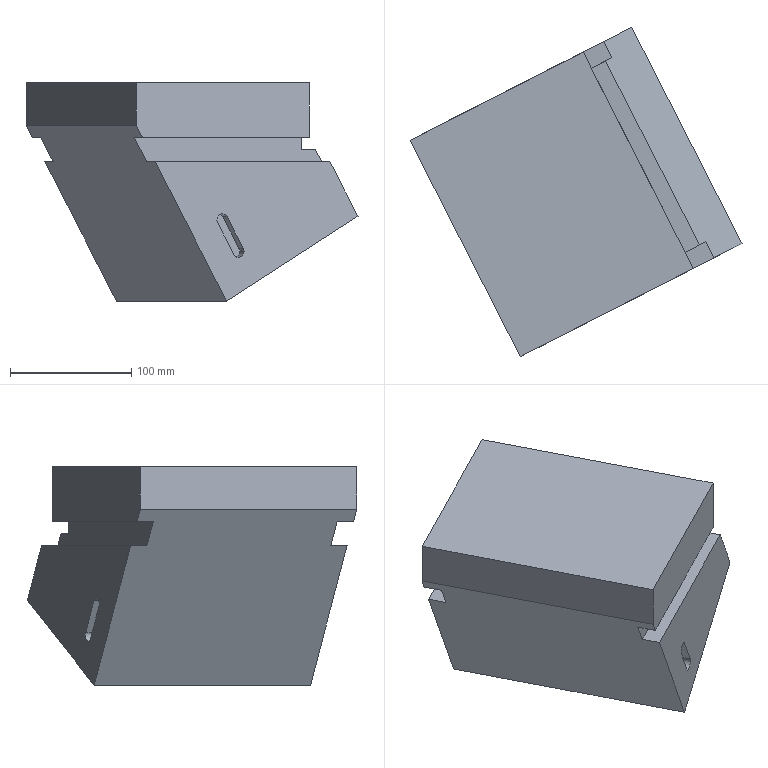Part | NX | features solid 2 | 1 solid | 27 faces | box 273.454 x 271.269 x 180 mm | volume 4546645 mm3 | plane 23 | cylinder 4 | commonest cylinder face diameters 10 x4
STEP:
#1=CARTESIAN_POINT('',(-1708.692,-455.362,180.));
#2=VERTEX_POINT('',#1);
#3=CARTESIAN_POINT('',(-1698.404,-450.119,160.));
#4=VERTEX_POINT('',#3);
#5=CARTESIAN_POINT('',(-1713.873,-458.001,190.07));
#6=DIRECTION('',(0.4455,0.227,-0.866));
#7=VECTOR('',#6,1000.);
#8=LINE('',#5,#7);
#9=EDGE_CURVE('',#2,#4,#8,.T.);
#10=ORIENTED_EDGE('',*,*,#9,.T.);
#11=CARTESIAN_POINT('',(-1705.214,-436.754,160.));
#12=VERTEX_POINT('',#11);
#13=CARTESIAN_POINT('',(-1614.416,-614.956,160.));
#14=DIRECTION('',(-0.454,0.891,0.));
#15=VECTOR('',#14,1000.);
#16=LINE('',#13,#15);
#17=EDGE_CURVE('',#4,#12,#16,.T.);
#18=ORIENTED_EDGE('',*,*,#17,.T.);
#19=CARTESIAN_POINT('',(-1646.055,-406.611,45.));
#20=VERTEX_POINT('',#19);
#21=CARTESIAN_POINT('',(-1720.683,-444.636,190.07));
#22=DIRECTION('',(0.4455,0.227,-0.866));
#23=VECTOR('',#22,1000.);
#24=LINE('',#21,#23);
#25=EDGE_CURVE('',#12,#20,#24,.T.);
#26=ORIENTED_EDGE('',*,*,#25,.T.);
#27=CARTESIAN_POINT('',(-1555.257,-584.813,45.));
#28=VERTEX_POINT('',#27);
#29=CARTESIAN_POINT('',(-1555.257,-584.813,45.));
#30=DIRECTION('',(-0.454,0.891,0.));
#31=VECTOR('',#30,1000.);
#32=LINE('',#29,#31);
#33=EDGE_CURVE('',#28,#20,#32,.T.);
#34=ORIENTED_EDGE('',*,*,#33,.F.);
#35=CARTESIAN_POINT('',(-1614.416,-614.956,160.));
#36=VERTEX_POINT('',#35);
#37=CARTESIAN_POINT('',(-1629.885,-622.837,190.07));
#38=DIRECTION('',(0.4455,0.227,-0.866));
#39=VECTOR('',#38,1000.);
#40=LINE('',#37,#39);
#41=EDGE_CURVE('',#36,#28,#40,.T.);
#42=ORIENTED_EDGE('',*,*,#41,.F.);
#43=CARTESIAN_POINT('',(-1621.226,-601.59,160.));
#44=VERTEX_POINT('',#43);
#45=CARTESIAN_POINT('',(-1614.416,-614.956,160.));
#46=DIRECTION('',(0.454,-0.891,0.));
#47=VECTOR('',#46,1000.);
#48=LINE('',#45,#47);
#49=EDGE_CURVE('',#44,#36,#48,.T.);
#50=ORIENTED_EDGE('',*,*,#49,.F.);
#51=CARTESIAN_POINT('',(-1631.514,-606.833,180.));
#52=VERTEX_POINT('',#51);
#53=CARTESIAN_POINT('',(-1636.694,-609.472,190.07));
#54=DIRECTION('',(0.4455,0.227,-0.866));
#55=VECTOR('',#54,1000.);
#56=LINE('',#53,#55);
#57=EDGE_CURVE('',#52,#44,#56,.T.);
#58=ORIENTED_EDGE('',*,*,#57,.F.);
#59=CARTESIAN_POINT('',(-1624.704,-620.198,180.));
#60=VERTEX_POINT('',#59);
#61=CARTESIAN_POINT('',(-1624.704,-620.198,180.));
#62=DIRECTION('',(0.454,-0.891,0.));
#63=VECTOR('',#62,1000.);
#64=LINE('',#61,#63);
#65=EDGE_CURVE('',#52,#60,#64,.T.);
#66=ORIENTED_EDGE('',*,*,#65,.T.);
#67=CARTESIAN_POINT('',(-1629.885,-622.837,190.07));
#68=VERTEX_POINT('',#67);
#69=CARTESIAN_POINT('',(-1629.885,-622.837,190.07));
#70=DIRECTION('',(0.4455,0.227,-0.866));
#71=VECTOR('',#70,1000.);
#72=LINE('',#69,#71);
#73=EDGE_CURVE('',#68,#60,#72,.T.);
#74=ORIENTED_EDGE('',*,*,#73,.F.);
#75=CARTESIAN_POINT('',(-1720.683,-444.636,190.07));
#76=VERTEX_POINT('',#75);
#77=CARTESIAN_POINT('',(-1629.885,-622.837,190.07));
#78=DIRECTION('',(-0.454,0.891,0.));
#79=VECTOR('',#78,1000.);
#80=LINE('',#77,#79);
#81=EDGE_CURVE('',#68,#76,#80,.T.);
#82=ORIENTED_EDGE('',*,*,#81,.T.);
#83=CARTESIAN_POINT('',(-1715.502,-441.996,180.));
#84=VERTEX_POINT('',#83);
#85=CARTESIAN_POINT('',(-1720.683,-444.636,190.07));
#86=DIRECTION('',(0.4455,0.227,-0.866));
#87=VECTOR('',#86,1000.);
#88=LINE('',#85,#87);
#89=EDGE_CURVE('',#76,#84,#88,.T.);
#90=ORIENTED_EDGE('',*,*,#89,.T.);
#91=CARTESIAN_POINT('',(-1624.704,-620.198,180.));
#92=DIRECTION('',(-0.454,0.891,0.));
#93=VECTOR('',#92,1000.);
#94=LINE('',#91,#93);
#95=EDGE_CURVE('',#2,#84,#94,.T.);
#96=ORIENTED_EDGE('',*,*,#95,.F.);
#97=EDGE_LOOP('',(#10,#18,#26,#34,#42,#50,#58,#66,#74,#82,#90,#96));
#98=FACE_BOUND('',#97,.T.);
#99=CARTESIAN_POINT('',(-1629.885,-622.837,190.07));
#100=DIRECTION('',(-0.7716,-0.3932,-0.5));
#101=DIRECTION('',(-0.4455,-0.227,0.866));
#102=AXIS2_PLACEMENT_3D('',#99,#100,#101);
#103=PLANE('',#102);
#104=ADVANCED_FACE('',(#98),#103,.T.);
#105=CARTESIAN_POINT('',(-1578.122,-371.998,180.));
#106=VERTEX_POINT('',#105);
#107=CARTESIAN_POINT('',(-1756.323,-462.796,180.));
#108=DIRECTION('',(0.891,0.454,0.));
#109=VECTOR('',#108,1000.);
#110=LINE('',#107,#109);
#111=EDGE_CURVE('',#84,#106,#110,.T.);
#112=ORIENTED_EDGE('',*,*,#111,.F.);
#113=ORIENTED_EDGE('',*,*,#89,.F.);
#114=CARTESIAN_POINT('',(-1720.683,-444.636,225.));
#115=VERTEX_POINT('',#114);
#116=CARTESIAN_POINT('',(-1720.683,-444.636,190.07));
#117=DIRECTION('',(0.,0.,1.));
#118=VECTOR('',#117,1000.);
#119=LINE('',#116,#118);
#120=EDGE_CURVE('',#76,#115,#119,.T.);
#121=ORIENTED_EDGE('',*,*,#120,.T.);
#122=CARTESIAN_POINT('',(-1578.122,-371.998,225.));
#123=VERTEX_POINT('',#122);
#124=CARTESIAN_POINT('',(-1720.683,-444.636,225.));
#125=DIRECTION('',(0.891,0.454,0.));
#126=VECTOR('',#125,1000.);
#127=LINE('',#124,#126);
#128=EDGE_CURVE('',#115,#123,#127,.T.);
#129=ORIENTED_EDGE('',*,*,#128,.T.);
#130=CARTESIAN_POINT('',(-1578.122,-371.998,170.));
#131=DIRECTION('',(0.,0.,1.));
#132=VECTOR('',#131,1000.);
#133=LINE('',#130,#132);
#134=EDGE_CURVE('',#106,#123,#133,.T.);
#135=ORIENTED_EDGE('',*,*,#134,.F.);
#136=EDGE_LOOP('',(#112,#113,#121,#129,#135));
#137=FACE_BOUND('',#136,.T.);
#138=CARTESIAN_POINT('',(-1720.683,-444.636,225.));
#139=DIRECTION('',(0.454,-0.891,0.));
#140=DIRECTION('',(0.,0.,1.));
#141=AXIS2_PLACEMENT_3D('',#138,#139,#140);
#142=PLANE('',#141);
#143=ADVANCED_FACE('',(#137),#142,.F.);
#144=CARTESIAN_POINT('',(-1571.312,-385.363,170.));
#145=VERTEX_POINT('',#144);
#146=CARTESIAN_POINT('',(-1571.312,-385.363,180.));
#147=VERTEX_POINT('',#146);
#148=CARTESIAN_POINT('',(-1571.312,-385.363,170.));
#149=DIRECTION('',(0.,0.,1.));
#150=VECTOR('',#149,1000.);
#151=LINE('',#148,#150);
#152=EDGE_CURVE('',#145,#147,#151,.T.);
#153=ORIENTED_EDGE('',*,*,#152,.T.);
#154=CARTESIAN_POINT('',(-1487.324,-550.199,180.));
#155=DIRECTION('',(0.454,-0.891,0.));
#156=VECTOR('',#155,1000.);
#157=LINE('',#154,#156);
#158=EDGE_CURVE('',#106,#147,#157,.T.);
#159=ORIENTED_EDGE('',*,*,#158,.F.);
#160=ORIENTED_EDGE('',*,*,#134,.T.);
#161=CARTESIAN_POINT('',(-1487.324,-550.199,225.));
#162=VERTEX_POINT('',#161);
#163=CARTESIAN_POINT('',(-1487.324,-550.199,225.));
#164=DIRECTION('',(-0.454,0.891,0.));
#165=VECTOR('',#164,1000.);
#166=LINE('',#163,#165);
#167=EDGE_CURVE('',#162,#123,#166,.T.);
#168=ORIENTED_EDGE('',*,*,#167,.F.);
#169=CARTESIAN_POINT('',(-1487.324,-550.199,180.));
#170=VERTEX_POINT('',#169);
#171=CARTESIAN_POINT('',(-1487.324,-550.199,170.));
#172=DIRECTION('',(0.,0.,1.));
#173=VECTOR('',#172,1000.);
#174=LINE('',#171,#173);
#175=EDGE_CURVE('',#170,#162,#174,.T.);
#176=ORIENTED_EDGE('',*,*,#175,.F.);
#177=CARTESIAN_POINT('',(-1494.133,-536.834,180.));
#178=VERTEX_POINT('',#177);
#179=CARTESIAN_POINT('',(-1487.324,-550.199,180.));
#180=DIRECTION('',(-0.454,0.891,0.));
#181=VECTOR('',#180,1000.);
#182=LINE('',#179,#181);
#183=EDGE_CURVE('',#170,#178,#182,.T.);
#184=ORIENTED_EDGE('',*,*,#183,.T.);
#185=CARTESIAN_POINT('',(-1494.133,-536.834,170.));
#186=VERTEX_POINT('',#185);
#187=CARTESIAN_POINT('',(-1494.133,-536.834,170.));
#188=DIRECTION('',(0.,0.,1.));
#189=VECTOR('',#188,1000.);
#190=LINE('',#187,#189);
#191=EDGE_CURVE('',#186,#178,#190,.T.);
#192=ORIENTED_EDGE('',*,*,#191,.F.);
#193=CARTESIAN_POINT('',(-1487.324,-550.199,170.));
#194=DIRECTION('',(-0.454,0.891,0.));
#195=VECTOR('',#194,1000.);
#196=LINE('',#193,#195);
#197=EDGE_CURVE('',#186,#145,#196,.T.);
#198=ORIENTED_EDGE('',*,*,#197,.T.);
#199=EDGE_LOOP('',(#153,#159,#160,#168,#176,#184,#192,#198));
#200=FACE_BOUND('',#199,.T.);
#201=CARTESIAN_POINT('',(-1487.324,-550.199,170.));
#202=DIRECTION('',(0.891,0.454,0.));
#203=DIRECTION('',(0.,0.,-1.));
#204=AXIS2_PLACEMENT_3D('',#201,#202,#203);
#205=PLANE('',#204);
#206=ADVANCED_FACE('',(#200),#205,.T.);
#207=CARTESIAN_POINT('',(-1559.51,-379.349,170.));
#208=VERTEX_POINT('',#207);
#209=CARTESIAN_POINT('',(-1559.51,-379.349,170.));
#210=DIRECTION('',(-0.891,-0.454,0.));
#211=VECTOR('',#210,1000.);
#212=LINE('',#209,#211);
#213=EDGE_CURVE('',#208,#145,#212,.T.);
#214=ORIENTED_EDGE('',*,*,#213,.T.);
#215=ORIENTED_EDGE('',*,*,#197,.F.);
#216=CARTESIAN_POINT('',(-1482.331,-530.82,170.));
#217=VERTEX_POINT('',#216);
#218=CARTESIAN_POINT('',(-1482.331,-530.82,170.));
#219=DIRECTION('',(-0.891,-0.454,0.));
#220=VECTOR('',#219,1000.);
#221=LINE('',#218,#220);
#222=EDGE_CURVE('',#217,#186,#221,.T.);
#223=ORIENTED_EDGE('',*,*,#222,.F.);
#224=CARTESIAN_POINT('',(-1475.521,-544.185,170.));
#225=DIRECTION('',(-0.454,0.891,0.));
#226=VECTOR('',#225,1000.);
#227=LINE('',#224,#226);
#228=EDGE_CURVE('',#217,#208,#227,.T.);
#229=ORIENTED_EDGE('',*,*,#228,.T.);
#230=EDGE_LOOP('',(#214,#215,#223,#229));
#231=FACE_BOUND('',#230,.T.);
#232=CARTESIAN_POINT('',(-1475.521,-544.185,170.));
#233=DIRECTION('',(0.,0.,1.));
#234=DIRECTION('',(0.891,0.454,0.));
#235=AXIS2_PLACEMENT_3D('',#232,#233,#234);
#236=PLANE('',#235);
#237=ADVANCED_FACE('',(#231),#236,.T.);
#238=CARTESIAN_POINT('',(-1554.365,-376.728,160.));
#239=VERTEX_POINT('',#238);
#240=CARTESIAN_POINT('',(-1531.216,-364.933,115.));
#241=DIRECTION('',(-0.4455,-0.227,0.866));
#242=VECTOR('',#241,1000.);
#243=LINE('',#240,#242);
#244=EDGE_CURVE('',#239,#208,#243,.T.);
#245=ORIENTED_EDGE('',*,*,#244,.T.);
#246=ORIENTED_EDGE('',*,*,#228,.F.);
#247=CARTESIAN_POINT('',(-1477.187,-528.199,160.));
#248=VERTEX_POINT('',#247);
#249=CARTESIAN_POINT('',(-1454.038,-516.404,115.));
#250=DIRECTION('',(-0.4455,-0.227,0.866));
#251=VECTOR('',#250,1000.);
#252=LINE('',#249,#251);
#253=EDGE_CURVE('',#248,#217,#252,.T.);
#254=ORIENTED_EDGE('',*,*,#253,.F.);
#255=CARTESIAN_POINT('',(-1470.377,-541.564,160.));
#256=VERTEX_POINT('',#255);
#257=CARTESIAN_POINT('',(-1470.377,-541.564,160.));
#258=DIRECTION('',(-0.454,0.891,0.));
#259=VECTOR('',#258,1000.);
#260=LINE('',#257,#259);
#261=EDGE_CURVE('',#256,#248,#260,.T.);
#262=ORIENTED_EDGE('',*,*,#261,.F.);
#263=CARTESIAN_POINT('',(-1447.228,-529.769,115.));
#264=VERTEX_POINT('',#263);
#265=CARTESIAN_POINT('',(-1447.228,-529.769,115.));
#266=DIRECTION('',(-0.4455,-0.227,0.866));
#267=VECTOR('',#266,1000.);
#268=LINE('',#265,#267);
#269=EDGE_CURVE('',#264,#256,#268,.T.);
#270=ORIENTED_EDGE('',*,*,#269,.F.);
#271=CARTESIAN_POINT('',(-1538.026,-351.568,115.));
#272=VERTEX_POINT('',#271);
#273=CARTESIAN_POINT('',(-1447.228,-529.769,115.));
#274=DIRECTION('',(-0.454,0.891,0.));
#275=VECTOR('',#274,1000.);
#276=LINE('',#273,#275);
#277=EDGE_CURVE('',#264,#272,#276,.T.);
#278=ORIENTED_EDGE('',*,*,#277,.T.);
#279=CARTESIAN_POINT('',(-1561.175,-363.363,160.));
#280=VERTEX_POINT('',#279);
#281=CARTESIAN_POINT('',(-1538.026,-351.568,115.));
#282=DIRECTION('',(-0.4455,-0.227,0.866));
#283=VECTOR('',#282,1000.);
#284=LINE('',#281,#283);
#285=EDGE_CURVE('',#272,#280,#284,.T.);
#286=ORIENTED_EDGE('',*,*,#285,.T.);
#287=CARTESIAN_POINT('',(-1470.377,-541.564,160.));
#288=DIRECTION('',(0.454,-0.891,0.));
#289=VECTOR('',#288,1000.);
#290=LINE('',#287,#289);
#291=EDGE_CURVE('',#280,#239,#290,.T.);
#292=ORIENTED_EDGE('',*,*,#291,.T.);
#293=EDGE_LOOP('',(#245,#246,#254,#262,#270,#278,#286,#292));
#294=FACE_BOUND('',#293,.T.);
#295=CARTESIAN_POINT('',(-1447.228,-529.769,115.));
#296=DIRECTION('',(0.7716,0.3932,0.5));
#297=DIRECTION('',(0.4455,0.227,-0.866));
#298=AXIS2_PLACEMENT_3D('',#295,#296,#297);
#299=PLANE('',#298);
#300=ADVANCED_FACE('',(#294),#299,.T.);
#301=CARTESIAN_POINT('',(-1541.701,-577.905,88.647));
#302=VERTEX_POINT('',#301);
#303=CARTESIAN_POINT('',(-1555.066,-584.715,114.628));
#304=VERTEX_POINT('',#303);
#305=CARTESIAN_POINT('',(-1548.383,-581.31,101.638));
#306=DIRECTION('',(-0.4455,-0.227,0.866));
#307=VECTOR('',#306,1000.);
#308=LINE('',#305,#307);
#309=EDGE_CURVE('',#302,#304,#308,.T.);
#310=ORIENTED_EDGE('',*,*,#309,.F.);
#311=CARTESIAN_POINT('',(-1549.417,-581.837,83.647));
#312=VERTEX_POINT('',#311);
#313=CARTESIAN_POINT('',(-1545.559,-579.871,86.147));
#314=DIRECTION('',(-0.454,0.891,0.));
#315=DIRECTION('',(0.,0.,1.));
#316=AXIS2_PLACEMENT_3D('',#313,#314,#315);
#317=CIRCLE('',#316,5.);
#318=EDGE_CURVE('',#302,#312,#317,.T.);
#319=ORIENTED_EDGE('',*,*,#318,.T.);
#320=CARTESIAN_POINT('',(-1562.782,-588.647,109.628));
#321=VERTEX_POINT('',#320);
#322=CARTESIAN_POINT('',(-1556.1,-585.242,96.638));
#323=DIRECTION('',(-0.4455,-0.227,0.866));
#324=VECTOR('',#323,1000.);
#325=LINE('',#322,#324);
#326=EDGE_CURVE('',#312,#321,#325,.T.);
#327=ORIENTED_EDGE('',*,*,#326,.T.);
#328=CARTESIAN_POINT('',(-1558.924,-586.681,112.128));
#329=DIRECTION('',(-0.454,0.891,0.));
#330=DIRECTION('',(0.,0.,1.));
#331=AXIS2_PLACEMENT_3D('',#328,#329,#330);
#332=CIRCLE('',#331,5.);
#333=EDGE_CURVE('',#321,#304,#332,.T.);
#334=ORIENTED_EDGE('',*,*,#333,.T.);
#335=EDGE_LOOP('',(#310,#319,#327,#334));
#336=FACE_BOUND('',#335,.T.);
#337=ORIENTED_EDGE('',*,*,#41,.T.);
#338=CARTESIAN_POINT('',(-1447.228,-529.769,115.));
#339=DIRECTION('',(-0.7716,-0.3932,-0.5));
#340=VECTOR('',#339,1000.);
#341=LINE('',#338,#340);
#342=EDGE_CURVE('',#264,#28,#341,.T.);
#343=ORIENTED_EDGE('',*,*,#342,.F.);
#344=ORIENTED_EDGE('',*,*,#269,.T.);
#345=CARTESIAN_POINT('',(-1665.525,-640.997,160.));
#346=DIRECTION('',(0.891,0.454,0.));
#347=VECTOR('',#346,1000.);
#348=LINE('',#345,#347);
#349=EDGE_CURVE('',#36,#256,#348,.T.);
#350=ORIENTED_EDGE('',*,*,#349,.F.);
#351=EDGE_LOOP('',(#337,#343,#344,#350));
#352=FACE_BOUND('',#351,.T.);
#353=CARTESIAN_POINT('',(-1629.885,-622.837,225.));
#354=DIRECTION('',(0.454,-0.891,0.));
#355=DIRECTION('',(0.,0.,1.));
#356=AXIS2_PLACEMENT_3D('',#353,#354,#355);
#357=PLANE('',#356);
#358=ADVANCED_FACE('',(#336,#352),#357,.T.);
#359=ORIENTED_EDGE('',*,*,#120,.F.);
#360=ORIENTED_EDGE('',*,*,#81,.F.);
#361=CARTESIAN_POINT('',(-1629.885,-622.837,225.));
#362=VERTEX_POINT('',#361);
#363=CARTESIAN_POINT('',(-1629.885,-622.837,190.07));
#364=DIRECTION('',(0.,0.,1.));
#365=VECTOR('',#364,1000.);
#366=LINE('',#363,#365);
#367=EDGE_CURVE('',#68,#362,#366,.T.);
#368=ORIENTED_EDGE('',*,*,#367,.T.);
#369=CARTESIAN_POINT('',(-1629.885,-622.837,225.));
#370=DIRECTION('',(-0.454,0.891,0.));
#371=VECTOR('',#370,1000.);
#372=LINE('',#369,#371);
#373=EDGE_CURVE('',#362,#115,#372,.T.);
#374=ORIENTED_EDGE('',*,*,#373,.T.);
#375=EDGE_LOOP('',(#359,#360,#368,#374));
#376=FACE_BOUND('',#375,.T.);
#377=CARTESIAN_POINT('',(-1629.885,-622.837,190.07));
#378=DIRECTION('',(0.891,0.454,0.));
#379=DIRECTION('',(0.,0.,-1.));
#380=AXIS2_PLACEMENT_3D('',#377,#378,#379);
#381=PLANE('',#380);
#382=ADVANCED_FACE('',(#376),#381,.F.);
#383=ORIENTED_EDGE('',*,*,#128,.F.);
#384=ORIENTED_EDGE('',*,*,#373,.F.);
#385=CARTESIAN_POINT('',(-1629.885,-622.837,225.));
#386=DIRECTION('',(0.891,0.454,0.));
#387=VECTOR('',#386,1000.);
#388=LINE('',#385,#387);
#389=EDGE_CURVE('',#362,#162,#388,.T.);
#390=ORIENTED_EDGE('',*,*,#389,.T.);
#391=ORIENTED_EDGE('',*,*,#167,.T.);
#392=EDGE_LOOP('',(#383,#384,#390,#391));
#393=FACE_BOUND('',#392,.T.);
#394=CARTESIAN_POINT('',(-1629.885,-622.837,225.));
#395=DIRECTION('',(0.,0.,-1.));
#396=DIRECTION('',(-0.891,-0.454,0.));
#397=AXIS2_PLACEMENT_3D('',#394,#395,#396);
#398=PLANE('',#397);
#399=ADVANCED_FACE('',(#393),#398,.F.);
#400=CARTESIAN_POINT('',(-1538.026,-351.568,115.));
#401=DIRECTION('',(-0.7716,-0.3932,-0.5));
#402=VECTOR('',#401,1000.);
#403=LINE('',#400,#402);
#404=EDGE_CURVE('',#272,#20,#403,.T.);
#405=ORIENTED_EDGE('',*,*,#404,.F.);
#406=ORIENTED_EDGE('',*,*,#277,.F.);
#407=ORIENTED_EDGE('',*,*,#342,.T.);
#408=ORIENTED_EDGE('',*,*,#33,.T.);
#409=EDGE_LOOP('',(#405,#406,#407,#408));
#410=FACE_BOUND('',#409,.T.);
#411=CARTESIAN_POINT('',(-1447.228,-529.769,115.));
#412=DIRECTION('',(-0.4455,-0.227,0.866));
#413=DIRECTION('',(0.7716,0.3932,0.5));
#414=AXIS2_PLACEMENT_3D('',#411,#412,#413);
#415=PLANE('',#414);
#416=ADVANCED_FACE('',(#410),#415,.F.);
#417=CARTESIAN_POINT('',(-1665.525,-640.997,180.));
#418=DIRECTION('',(0.891,0.454,0.));
#419=VECTOR('',#418,1000.);
#420=LINE('',#417,#419);
#421=EDGE_CURVE('',#60,#170,#420,.T.);
#422=ORIENTED_EDGE('',*,*,#421,.T.);
#423=ORIENTED_EDGE('',*,*,#175,.T.);
#424=ORIENTED_EDGE('',*,*,#389,.F.);
#425=ORIENTED_EDGE('',*,*,#367,.F.);
#426=ORIENTED_EDGE('',*,*,#73,.T.);
#427=EDGE_LOOP('',(#422,#423,#424,#425,#426));
#428=FACE_BOUND('',#427,.T.);
#429=CARTESIAN_POINT('',(-1629.885,-622.837,225.));
#430=DIRECTION('',(0.454,-0.891,0.));
#431=DIRECTION('',(0.,0.,1.));
#432=AXIS2_PLACEMENT_3D('',#429,#430,#431);
#433=PLANE('',#432);
#434=ADVANCED_FACE('',(#428),#433,.T.);
#435=CARTESIAN_POINT('',(-1645.864,-406.514,114.628));
#436=VERTEX_POINT('',#435);
#437=CARTESIAN_POINT('',(-1653.58,-410.446,109.628));
#438=VERTEX_POINT('',#437);
#439=CARTESIAN_POINT('',(-1649.722,-408.48,112.128));
#440=DIRECTION('',(0.454,-0.891,0.));
#441=DIRECTION('',(0.,0.,-1.));
#442=AXIS2_PLACEMENT_3D('',#439,#440,#441);
#443=CIRCLE('',#442,5.);
#444=EDGE_CURVE('',#436,#438,#443,.T.);
#445=ORIENTED_EDGE('',*,*,#444,.T.);
#446=CARTESIAN_POINT('',(-1640.215,-403.636,83.647));
#447=VERTEX_POINT('',#446);
#448=CARTESIAN_POINT('',(-1646.898,-407.041,96.638));
#449=DIRECTION('',(0.4455,0.227,-0.866));
#450=VECTOR('',#449,1000.);
#451=LINE('',#448,#450);
#452=EDGE_CURVE('',#438,#447,#451,.T.);
#453=ORIENTED_EDGE('',*,*,#452,.T.);
#454=CARTESIAN_POINT('',(-1632.499,-399.704,88.647));
#455=VERTEX_POINT('',#454);
#456=CARTESIAN_POINT('',(-1636.357,-401.67,86.147));
#457=DIRECTION('',(0.454,-0.891,0.));
#458=DIRECTION('',(0.,0.,-1.));
#459=AXIS2_PLACEMENT_3D('',#456,#457,#458);
#460=CIRCLE('',#459,5.);
#461=EDGE_CURVE('',#447,#455,#460,.T.);
#462=ORIENTED_EDGE('',*,*,#461,.T.);
#463=CARTESIAN_POINT('',(-1639.181,-403.109,101.638));
#464=DIRECTION('',(0.4455,0.227,-0.866));
#465=VECTOR('',#464,1000.);
#466=LINE('',#463,#465);
#467=EDGE_CURVE('',#436,#455,#466,.T.);
#468=ORIENTED_EDGE('',*,*,#467,.F.);
#469=EDGE_LOOP('',(#445,#453,#462,#468));
#470=FACE_BOUND('',#469,.T.);
#471=ORIENTED_EDGE('',*,*,#285,.F.);
#472=ORIENTED_EDGE('',*,*,#404,.T.);
#473=ORIENTED_EDGE('',*,*,#25,.F.);
#474=CARTESIAN_POINT('',(-1756.323,-462.796,160.));
#475=DIRECTION('',(0.891,0.454,0.));
#476=VECTOR('',#475,1000.);
#477=LINE('',#474,#476);
#478=EDGE_CURVE('',#12,#280,#477,.T.);
#479=ORIENTED_EDGE('',*,*,#478,.T.);
#480=EDGE_LOOP('',(#471,#472,#473,#479));
#481=FACE_BOUND('',#480,.T.);
#482=CARTESIAN_POINT('',(-1720.683,-444.636,225.));
#483=DIRECTION('',(0.454,-0.891,0.));
#484=DIRECTION('',(0.,0.,1.));
#485=AXIS2_PLACEMENT_3D('',#482,#483,#484);
#486=PLANE('',#485);
#487=ADVANCED_FACE('',(#470,#481),#486,.F.);
#488=ORIENTED_EDGE('',*,*,#467,.T.);
#489=CARTESIAN_POINT('',(-1628.867,-406.832,88.647));
#490=VERTEX_POINT('',#489);
#491=CARTESIAN_POINT('',(-1632.499,-399.704,88.647));
#492=DIRECTION('',(-0.454,0.891,0.));
#493=VECTOR('',#492,1000.);
#494=LINE('',#491,#493);
#495=EDGE_CURVE('',#490,#455,#494,.T.);
#496=ORIENTED_EDGE('',*,*,#495,.F.);
#497=CARTESIAN_POINT('',(-1642.232,-413.642,114.628));
#498=VERTEX_POINT('',#497);
#499=CARTESIAN_POINT('',(-1642.232,-413.642,114.628));
#500=DIRECTION('',(0.4455,0.227,-0.866));
#501=VECTOR('',#500,1000.);
#502=LINE('',#499,#501);
#503=EDGE_CURVE('',#498,#490,#502,.T.);
#504=ORIENTED_EDGE('',*,*,#503,.F.);
#505=CARTESIAN_POINT('',(-1645.864,-406.514,114.628));
#506=DIRECTION('',(-0.454,0.891,0.));
#507=VECTOR('',#506,1000.);
#508=LINE('',#505,#507);
#509=EDGE_CURVE('',#498,#436,#508,.T.);
#510=ORIENTED_EDGE('',*,*,#509,.T.);
#511=EDGE_LOOP('',(#488,#496,#504,#510));
#512=FACE_BOUND('',#511,.T.);
#513=CARTESIAN_POINT('',(-1639.181,-403.109,101.638));
#514=DIRECTION('',(0.7716,0.3932,0.5));
#515=DIRECTION('',(0.4455,0.227,-0.866));
#516=AXIS2_PLACEMENT_3D('',#513,#514,#515);
#517=PLANE('',#516);
#518=ADVANCED_FACE('',(#512),#517,.F.);
#519=ORIENTED_EDGE('',*,*,#503,.T.);
#520=CARTESIAN_POINT('',(-1636.583,-410.764,83.647));
#521=VERTEX_POINT('',#520);
#522=CARTESIAN_POINT('',(-1632.725,-408.798,86.147));
#523=DIRECTION('',(0.454,-0.891,0.));
#524=DIRECTION('',(0.,0.,-1.));
#525=AXIS2_PLACEMENT_3D('',#522,#523,#524);
#526=CIRCLE('',#525,5.);
#527=EDGE_CURVE('',#521,#490,#526,.T.);
#528=ORIENTED_EDGE('',*,*,#527,.F.);
#529=CARTESIAN_POINT('',(-1649.948,-417.574,109.628));
#530=VERTEX_POINT('',#529);
#531=CARTESIAN_POINT('',(-1649.948,-417.574,109.628));
#532=DIRECTION('',(0.4455,0.227,-0.866));
#533=VECTOR('',#532,1000.);
#534=LINE('',#531,#533);
#535=EDGE_CURVE('',#530,#521,#534,.T.);
#536=ORIENTED_EDGE('',*,*,#535,.F.);
#537=CARTESIAN_POINT('',(-1646.09,-415.608,112.128));
#538=DIRECTION('',(0.454,-0.891,0.));
#539=DIRECTION('',(0.,0.,-1.));
#540=AXIS2_PLACEMENT_3D('',#537,#538,#539);
#541=CIRCLE('',#540,5.);
#542=EDGE_CURVE('',#498,#530,#541,.T.);
#543=ORIENTED_EDGE('',*,*,#542,.F.);
#544=EDGE_LOOP('',(#519,#528,#536,#543));
#545=FACE_BOUND('',#544,.T.);
#546=CARTESIAN_POINT('',(-1639.408,-412.203,99.138));
#547=DIRECTION('',(0.454,-0.891,0.));
#548=DIRECTION('',(0.,0.,1.));
#549=AXIS2_PLACEMENT_3D('',#546,#547,#548);
#550=PLANE('',#549);
#551=ADVANCED_FACE('',(#545),#550,.F.);
#552=ORIENTED_EDGE('',*,*,#444,.F.);
#553=ORIENTED_EDGE('',*,*,#509,.F.);
#554=ORIENTED_EDGE('',*,*,#542,.T.);
#555=CARTESIAN_POINT('',(-1653.58,-410.446,109.628));
#556=DIRECTION('',(-0.454,0.891,0.));
#557=VECTOR('',#556,1000.);
#558=LINE('',#555,#557);
#559=EDGE_CURVE('',#530,#438,#558,.T.);
#560=ORIENTED_EDGE('',*,*,#559,.T.);
#561=EDGE_LOOP('',(#552,#553,#554,#560));
#562=FACE_BOUND('',#561,.T.);
#563=CARTESIAN_POINT('',(-1649.722,-408.48,112.128));
#564=DIRECTION('',(-0.454,0.891,0.));
#565=DIRECTION('',(0.,0.,-1.));
#566=AXIS2_PLACEMENT_3D('',#563,#564,#565);
#567=CYLINDRICAL_SURFACE('',#566,5.);
#568=ADVANCED_FACE('',(#562),#567,.F.);
#569=ORIENTED_EDGE('',*,*,#452,.F.);
#570=ORIENTED_EDGE('',*,*,#559,.F.);
#571=ORIENTED_EDGE('',*,*,#535,.T.);
#572=CARTESIAN_POINT('',(-1640.215,-403.636,83.647));
#573=DIRECTION('',(-0.454,0.891,0.));
#574=VECTOR('',#573,1000.);
#575=LINE('',#572,#574);
#576=EDGE_CURVE('',#521,#447,#575,.T.);
#577=ORIENTED_EDGE('',*,*,#576,.T.);
#578=EDGE_LOOP('',(#569,#570,#571,#577));
#579=FACE_BOUND('',#578,.T.);
#580=CARTESIAN_POINT('',(-1646.898,-407.041,96.638));
#581=DIRECTION('',(-0.7716,-0.3932,-0.5));
#582=DIRECTION('',(-0.4455,-0.227,0.866));
#583=AXIS2_PLACEMENT_3D('',#580,#581,#582);
#584=PLANE('',#583);
#585=ADVANCED_FACE('',(#579),#584,.F.);
#586=ORIENTED_EDGE('',*,*,#461,.F.);
#587=ORIENTED_EDGE('',*,*,#576,.F.);
#588=ORIENTED_EDGE('',*,*,#527,.T.);
#589=ORIENTED_EDGE('',*,*,#495,.T.);
#590=EDGE_LOOP('',(#586,#587,#588,#589));
#591=FACE_BOUND('',#590,.T.);
#592=CARTESIAN_POINT('',(-1636.357,-401.67,86.147));
#593=DIRECTION('',(-0.454,0.891,0.));
#594=DIRECTION('',(0.,0.,-1.));
#595=AXIS2_PLACEMENT_3D('',#592,#593,#594);
#596=CYLINDRICAL_SURFACE('',#595,5.);
#597=ADVANCED_FACE('',(#591),#596,.F.);
#598=ORIENTED_EDGE('',*,*,#309,.T.);
#599=CARTESIAN_POINT('',(-1558.698,-577.587,114.628));
#600=VERTEX_POINT('',#599);
#601=CARTESIAN_POINT('',(-1555.066,-584.715,114.628));
#602=DIRECTION('',(0.454,-0.891,0.));
#603=VECTOR('',#602,1000.);
#604=LINE('',#601,#603);
#605=EDGE_CURVE('',#600,#304,#604,.T.);
#606=ORIENTED_EDGE('',*,*,#605,.F.);
#607=CARTESIAN_POINT('',(-1545.333,-570.777,88.647));
#608=VERTEX_POINT('',#607);
#609=CARTESIAN_POINT('',(-1545.333,-570.777,88.647));
#610=DIRECTION('',(-0.4455,-0.227,0.866));
#611=VECTOR('',#610,1000.);
#612=LINE('',#609,#611);
#613=EDGE_CURVE('',#608,#600,#612,.T.);
#614=ORIENTED_EDGE('',*,*,#613,.F.);
#615=CARTESIAN_POINT('',(-1541.701,-577.905,88.647));
#616=DIRECTION('',(0.454,-0.891,0.));
#617=VECTOR('',#616,1000.);
#618=LINE('',#615,#617);
#619=EDGE_CURVE('',#608,#302,#618,.T.);
#620=ORIENTED_EDGE('',*,*,#619,.T.);
#621=EDGE_LOOP('',(#598,#606,#614,#620));
#622=FACE_BOUND('',#621,.T.);
#623=CARTESIAN_POINT('',(-1548.383,-581.31,101.638));
#624=DIRECTION('',(0.7716,0.3932,0.5));
#625=DIRECTION('',(0.4455,0.227,-0.866));
#626=AXIS2_PLACEMENT_3D('',#623,#624,#625);
#627=PLANE('',#626);
#628=ADVANCED_FACE('',(#622),#627,.F.);
#629=ORIENTED_EDGE('',*,*,#613,.T.);
#630=CARTESIAN_POINT('',(-1566.414,-581.519,109.628));
#631=VERTEX_POINT('',#630);
#632=CARTESIAN_POINT('',(-1562.556,-579.553,112.128));
#633=DIRECTION('',(-0.454,0.891,0.));
#634=DIRECTION('',(0.,0.,1.));
#635=AXIS2_PLACEMENT_3D('',#632,#633,#634);
#636=CIRCLE('',#635,5.);
#637=EDGE_CURVE('',#631,#600,#636,.T.);
#638=ORIENTED_EDGE('',*,*,#637,.F.);
#639=CARTESIAN_POINT('',(-1553.049,-574.709,83.647));
#640=VERTEX_POINT('',#639);
#641=CARTESIAN_POINT('',(-1553.049,-574.709,83.647));
#642=DIRECTION('',(-0.4455,-0.227,0.866));
#643=VECTOR('',#642,1000.);
#644=LINE('',#641,#643);
#645=EDGE_CURVE('',#640,#631,#644,.T.);
#646=ORIENTED_EDGE('',*,*,#645,.F.);
#647=CARTESIAN_POINT('',(-1549.191,-572.743,86.147));
#648=DIRECTION('',(-0.454,0.891,0.));
#649=DIRECTION('',(0.,0.,1.));
#650=AXIS2_PLACEMENT_3D('',#647,#648,#649);
#651=CIRCLE('',#650,5.);
#652=EDGE_CURVE('',#608,#640,#651,.T.);
#653=ORIENTED_EDGE('',*,*,#652,.F.);
#654=EDGE_LOOP('',(#629,#638,#646,#653));
#655=FACE_BOUND('',#654,.T.);
#656=CARTESIAN_POINT('',(-1555.873,-576.148,99.138));
#657=DIRECTION('',(-0.454,0.891,0.));
#658=DIRECTION('',(0.,0.,-1.));
#659=AXIS2_PLACEMENT_3D('',#656,#657,#658);
#660=PLANE('',#659);
#661=ADVANCED_FACE('',(#655),#660,.F.);
#662=ORIENTED_EDGE('',*,*,#318,.F.);
#663=ORIENTED_EDGE('',*,*,#619,.F.);
#664=ORIENTED_EDGE('',*,*,#652,.T.);
#665=CARTESIAN_POINT('',(-1549.417,-581.837,83.647));
#666=DIRECTION('',(0.454,-0.891,0.));
#667=VECTOR('',#666,1000.);
#668=LINE('',#665,#667);
#669=EDGE_CURVE('',#640,#312,#668,.T.);
#670=ORIENTED_EDGE('',*,*,#669,.T.);
#671=EDGE_LOOP('',(#662,#663,#664,#670));
#672=FACE_BOUND('',#671,.T.);
#673=CARTESIAN_POINT('',(-1545.559,-579.871,86.147));
#674=DIRECTION('',(0.454,-0.891,0.));
#675=DIRECTION('',(0.,0.,1.));
#676=AXIS2_PLACEMENT_3D('',#673,#674,#675);
#677=CYLINDRICAL_SURFACE('',#676,5.);
#678=ADVANCED_FACE('',(#672),#677,.F.);
#679=ORIENTED_EDGE('',*,*,#326,.F.);
#680=ORIENTED_EDGE('',*,*,#669,.F.);
#681=ORIENTED_EDGE('',*,*,#645,.T.);
#682=CARTESIAN_POINT('',(-1562.782,-588.647,109.628));
#683=DIRECTION('',(0.454,-0.891,0.));
#684=VECTOR('',#683,1000.);
#685=LINE('',#682,#684);
#686=EDGE_CURVE('',#631,#321,#685,.T.);
#687=ORIENTED_EDGE('',*,*,#686,.T.);
#688=EDGE_LOOP('',(#679,#680,#681,#687));
#689=FACE_BOUND('',#688,.T.);
#690=CARTESIAN_POINT('',(-1556.1,-585.242,96.638));
#691=DIRECTION('',(-0.7716,-0.3932,-0.5));
#692=DIRECTION('',(-0.4455,-0.227,0.866));
#693=AXIS2_PLACEMENT_3D('',#690,#691,#692);
#694=PLANE('',#693);
#695=ADVANCED_FACE('',(#689),#694,.F.);
#696=ORIENTED_EDGE('',*,*,#333,.F.);
#697=ORIENTED_EDGE('',*,*,#686,.F.);
#698=ORIENTED_EDGE('',*,*,#637,.T.);
#699=ORIENTED_EDGE('',*,*,#605,.T.);
#700=EDGE_LOOP('',(#696,#697,#698,#699));
#701=FACE_BOUND('',#700,.T.);
#702=CARTESIAN_POINT('',(-1558.924,-586.681,112.128));
#703=DIRECTION('',(0.454,-0.891,0.));
#704=DIRECTION('',(0.,0.,1.));
#705=AXIS2_PLACEMENT_3D('',#702,#703,#704);
#706=CYLINDRICAL_SURFACE('',#705,5.);
#707=ADVANCED_FACE('',(#701),#706,.F.);
#708=ORIENTED_EDGE('',*,*,#349,.T.);
#709=ORIENTED_EDGE('',*,*,#261,.T.);
#710=CARTESIAN_POINT('',(-1672.335,-627.632,160.));
#711=DIRECTION('',(0.891,0.454,0.));
#712=VECTOR('',#711,1000.);
#713=LINE('',#710,#712);
#714=EDGE_CURVE('',#44,#248,#713,.T.);
#715=ORIENTED_EDGE('',*,*,#714,.F.);
#716=ORIENTED_EDGE('',*,*,#49,.T.);
#717=EDGE_LOOP('',(#708,#709,#715,#716));
#718=FACE_BOUND('',#717,.T.);
#719=CARTESIAN_POINT('',(-1665.525,-640.997,160.));
#720=DIRECTION('',(0.,0.,1.));
#721=DIRECTION('',(0.891,0.454,0.));
#722=AXIS2_PLACEMENT_3D('',#719,#720,#721);
#723=PLANE('',#722);
#724=ADVANCED_FACE('',(#718),#723,.T.);
#725=ORIENTED_EDGE('',*,*,#222,.T.);
#726=ORIENTED_EDGE('',*,*,#191,.T.);
#727=CARTESIAN_POINT('',(-1672.335,-627.632,180.));
#728=DIRECTION('',(0.891,0.454,0.));
#729=VECTOR('',#728,1000.);
#730=LINE('',#727,#729);
#731=EDGE_CURVE('',#52,#178,#730,.T.);
#732=ORIENTED_EDGE('',*,*,#731,.F.);
#733=ORIENTED_EDGE('',*,*,#57,.T.);
#734=ORIENTED_EDGE('',*,*,#714,.T.);
#735=ORIENTED_EDGE('',*,*,#253,.T.);
#736=EDGE_LOOP('',(#725,#726,#732,#733,#734,#735));
#737=FACE_BOUND('',#736,.T.);
#738=CARTESIAN_POINT('',(-1672.335,-627.632,160.));
#739=DIRECTION('',(0.454,-0.891,0.));
#740=DIRECTION('',(0.,0.,1.));
#741=AXIS2_PLACEMENT_3D('',#738,#739,#740);
#742=PLANE('',#741);
#743=ADVANCED_FACE('',(#737),#742,.T.);
#744=ORIENTED_EDGE('',*,*,#183,.F.);
#745=ORIENTED_EDGE('',*,*,#421,.F.);
#746=ORIENTED_EDGE('',*,*,#65,.F.);
#747=ORIENTED_EDGE('',*,*,#731,.T.);
#748=EDGE_LOOP('',(#744,#745,#746,#747));
#749=FACE_BOUND('',#748,.T.);
#750=CARTESIAN_POINT('',(-1665.525,-640.997,180.));
#751=DIRECTION('',(0.,0.,1.));
#752=DIRECTION('',(0.891,0.454,0.));
#753=AXIS2_PLACEMENT_3D('',#750,#751,#752);
#754=PLANE('',#753);
#755=ADVANCED_FACE('',(#749),#754,.F.);
#756=ORIENTED_EDGE('',*,*,#152,.F.);
#757=ORIENTED_EDGE('',*,*,#213,.F.);
#758=ORIENTED_EDGE('',*,*,#244,.F.);
#759=CARTESIAN_POINT('',(-1749.513,-476.161,160.));
#760=DIRECTION('',(0.891,0.454,0.));
#761=VECTOR('',#760,1000.);
#762=LINE('',#759,#761);
#763=EDGE_CURVE('',#4,#239,#762,.T.);
#764=ORIENTED_EDGE('',*,*,#763,.F.);
#765=ORIENTED_EDGE('',*,*,#9,.F.);
#766=CARTESIAN_POINT('',(-1749.513,-476.161,180.));
#767=DIRECTION('',(0.891,0.454,0.));
#768=VECTOR('',#767,1000.);
#769=LINE('',#766,#768);
#770=EDGE_CURVE('',#2,#147,#769,.T.);
#771=ORIENTED_EDGE('',*,*,#770,.T.);
#772=EDGE_LOOP('',(#756,#757,#758,#764,#765,#771));
#773=FACE_BOUND('',#772,.T.);
#774=CARTESIAN_POINT('',(-1749.513,-476.161,160.));
#775=DIRECTION('',(0.454,-0.891,0.));
#776=DIRECTION('',(0.,0.,1.));
#777=AXIS2_PLACEMENT_3D('',#774,#775,#776);
#778=PLANE('',#777);
#779=ADVANCED_FACE('',(#773),#778,.F.);
#780=ORIENTED_EDGE('',*,*,#111,.T.);
#781=ORIENTED_EDGE('',*,*,#158,.T.);
#782=ORIENTED_EDGE('',*,*,#770,.F.);
#783=ORIENTED_EDGE('',*,*,#95,.T.);
#784=EDGE_LOOP('',(#780,#781,#782,#783));
#785=FACE_BOUND('',#784,.T.);
#786=CARTESIAN_POINT('',(-1756.323,-462.796,180.));
#787=DIRECTION('',(0.,0.,-1.));
#788=DIRECTION('',(-0.891,-0.454,0.));
#789=AXIS2_PLACEMENT_3D('',#786,#787,#788);
#790=PLANE('',#789);
#791=ADVANCED_FACE('',(#785),#790,.T.);
#792=ORIENTED_EDGE('',*,*,#291,.F.);
#793=ORIENTED_EDGE('',*,*,#478,.F.);
#794=ORIENTED_EDGE('',*,*,#17,.F.);
#795=ORIENTED_EDGE('',*,*,#763,.T.);
#796=EDGE_LOOP('',(#792,#793,#794,#795));
#797=FACE_BOUND('',#796,.T.);
#798=CARTESIAN_POINT('',(-1756.323,-462.796,160.));
#799=DIRECTION('',(0.,0.,-1.));
#800=DIRECTION('',(-0.891,-0.454,0.));
#801=AXIS2_PLACEMENT_3D('',#798,#799,#800);
#802=PLANE('',#801);
#803=ADVANCED_FACE('',(#797),#802,.F.);
#804=CLOSED_SHELL('',(#104,#143,#206,#237,#300,#358,#382,#399,#416,#434,#487,#518,#551,#568,#585,#597,#628,#661,#678,#695,#707,#724,#743,#755,#779,#791,#803));
#805=MANIFOLD_SOLID_BREP('',#804);
#806=(LENGTH_UNIT()NAMED_UNIT(*)SI_UNIT(.MILLI.,.METRE.));
#807=UNCERTAINTY_MEASURE_WITH_UNIT(LENGTH_MEASURE(0.00001),#806,'','');
#808=(NAMED_UNIT(*)PLANE_ANGLE_UNIT()SI_UNIT($,.RADIAN.));
#809=(NAMED_UNIT(*)SI_UNIT($,.STERADIAN.)SOLID_ANGLE_UNIT());
#810=(GEOMETRIC_REPRESENTATION_CONTEXT(3)GLOBAL_UNCERTAINTY_ASSIGNED_CONTEXT((#807))GLOBAL_UNIT_ASSIGNED_CONTEXT((#806,#808,#809))REPRESENTATION_CONTEXT('',''));
#811=ADVANCED_BREP_SHAPE_REPRESENTATION('',(#805),#810);